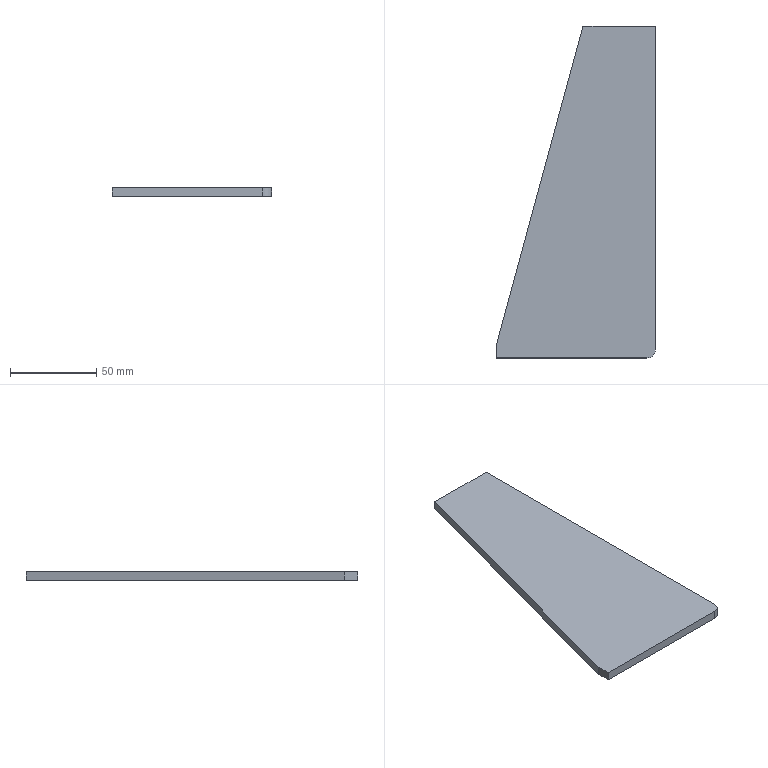Part | SolidWorks | features Extrusion 1 | 1 solid | 8 faces | box 92 x 192 x 5 mm | volume 65293 mm3 | plane 7 | cylinder 1 | commonest cylinder face diameters 10 x1
STEP:
#1=CARTESIAN_POINT('',(42.,-187.,0.));
#2=VERTEX_POINT('',#1);
#3=CARTESIAN_POINT('',(42.,0.,0.));
#4=VERTEX_POINT('',#3);
#5=CARTESIAN_POINT('',(42.,-187.,0.));
#6=DIRECTION('',(0.,1.,0.));
#7=VECTOR('',#6,1000.);
#8=LINE('',#5,#7);
#9=EDGE_CURVE('',#2,#4,#8,.T.);
#10=ORIENTED_EDGE('',*,*,#9,.T.);
#11=CARTESIAN_POINT('',(42.,0.,5.));
#12=VERTEX_POINT('',#11);
#13=CARTESIAN_POINT('',(42.,0.,5.));
#14=DIRECTION('',(0.,0.,-1.));
#15=VECTOR('',#14,1000.);
#16=LINE('',#13,#15);
#17=EDGE_CURVE('',#12,#4,#16,.T.);
#18=ORIENTED_EDGE('',*,*,#17,.F.);
#19=CARTESIAN_POINT('',(42.,-187.,5.));
#20=VERTEX_POINT('',#19);
#21=CARTESIAN_POINT('',(42.,-187.,5.));
#22=DIRECTION('',(0.,1.,0.));
#23=VECTOR('',#22,1000.);
#24=LINE('',#21,#23);
#25=EDGE_CURVE('',#20,#12,#24,.T.);
#26=ORIENTED_EDGE('',*,*,#25,.F.);
#27=CARTESIAN_POINT('',(42.,-187.,5.));
#28=DIRECTION('',(0.,0.,-1.));
#29=VECTOR('',#28,1000.);
#30=LINE('',#27,#29);
#31=EDGE_CURVE('',#20,#2,#30,.T.);
#32=ORIENTED_EDGE('',*,*,#31,.T.);
#33=EDGE_LOOP('',(#10,#18,#26,#32));
#34=FACE_OUTER_BOUND('',#33,.T.);
#35=CARTESIAN_POINT('',(42.,-187.,5.));
#36=DIRECTION('',(-1.,0.,0.));
#37=DIRECTION('',(0.,0.,1.));
#38=AXIS2_PLACEMENT_3D('',#35,#36,#37);
#39=PLANE('',#38);
#40=ADVANCED_FACE('',(#34),#39,.F.);
#41=CARTESIAN_POINT('',(0.,0.,0.));
#42=VERTEX_POINT('',#41);
#43=CARTESIAN_POINT('',(42.,0.,0.));
#44=DIRECTION('',(-1.,0.,0.));
#45=VECTOR('',#44,1000.);
#46=LINE('',#43,#45);
#47=EDGE_CURVE('',#4,#42,#46,.T.);
#48=ORIENTED_EDGE('',*,*,#47,.T.);
#49=CARTESIAN_POINT('',(0.,0.,5.));
#50=VERTEX_POINT('',#49);
#51=CARTESIAN_POINT('',(0.,0.,5.));
#52=DIRECTION('',(0.,0.,-1.));
#53=VECTOR('',#52,1000.);
#54=LINE('',#51,#53);
#55=EDGE_CURVE('',#50,#42,#54,.T.);
#56=ORIENTED_EDGE('',*,*,#55,.F.);
#57=CARTESIAN_POINT('',(42.,0.,5.));
#58=DIRECTION('',(-1.,0.,0.));
#59=VECTOR('',#58,1000.);
#60=LINE('',#57,#59);
#61=EDGE_CURVE('',#12,#50,#60,.T.);
#62=ORIENTED_EDGE('',*,*,#61,.F.);
#63=ORIENTED_EDGE('',*,*,#17,.T.);
#64=EDGE_LOOP('',(#48,#56,#62,#63));
#65=FACE_OUTER_BOUND('',#64,.T.);
#66=CARTESIAN_POINT('',(42.,0.,5.));
#67=DIRECTION('',(0.,-1.,0.));
#68=DIRECTION('',(0.,0.,-1.));
#69=AXIS2_PLACEMENT_3D('',#66,#67,#68);
#70=PLANE('',#69);
#71=ADVANCED_FACE('',(#65),#70,.F.);
#72=CARTESIAN_POINT('',(-50.,-184.,0.));
#73=VERTEX_POINT('',#72);
#74=CARTESIAN_POINT('',(0.,0.,0.));
#75=DIRECTION('',(-0.2622,-0.965,0.));
#76=VECTOR('',#75,1000.);
#77=LINE('',#74,#76);
#78=EDGE_CURVE('',#42,#73,#77,.T.);
#79=ORIENTED_EDGE('',*,*,#78,.T.);
#80=CARTESIAN_POINT('',(-50.,-184.,5.));
#81=VERTEX_POINT('',#80);
#82=CARTESIAN_POINT('',(-50.,-184.,5.));
#83=DIRECTION('',(0.,0.,-1.));
#84=VECTOR('',#83,1000.);
#85=LINE('',#82,#84);
#86=EDGE_CURVE('',#81,#73,#85,.T.);
#87=ORIENTED_EDGE('',*,*,#86,.F.);
#88=CARTESIAN_POINT('',(0.,0.,5.));
#89=DIRECTION('',(-0.2622,-0.965,0.));
#90=VECTOR('',#89,1000.);
#91=LINE('',#88,#90);
#92=EDGE_CURVE('',#50,#81,#91,.T.);
#93=ORIENTED_EDGE('',*,*,#92,.F.);
#94=ORIENTED_EDGE('',*,*,#55,.T.);
#95=EDGE_LOOP('',(#79,#87,#93,#94));
#96=FACE_OUTER_BOUND('',#95,.T.);
#97=CARTESIAN_POINT('',(0.,0.,5.));
#98=DIRECTION('',(0.965,-0.2622,0.));
#99=DIRECTION('',(0.2622,0.965,0.));
#100=AXIS2_PLACEMENT_3D('',#97,#98,#99);
#101=PLANE('',#100);
#102=ADVANCED_FACE('',(#96),#101,.F.);
#103=CARTESIAN_POINT('',(-50.,-192.,0.));
#104=VERTEX_POINT('',#103);
#105=CARTESIAN_POINT('',(-50.,-184.,0.));
#106=DIRECTION('',(0.,-1.,0.));
#107=VECTOR('',#106,1000.);
#108=LINE('',#105,#107);
#109=EDGE_CURVE('',#73,#104,#108,.T.);
#110=ORIENTED_EDGE('',*,*,#109,.T.);
#111=CARTESIAN_POINT('',(-50.,-192.,5.));
#112=VERTEX_POINT('',#111);
#113=CARTESIAN_POINT('',(-50.,-192.,5.));
#114=DIRECTION('',(0.,0.,-1.));
#115=VECTOR('',#114,1000.);
#116=LINE('',#113,#115);
#117=EDGE_CURVE('',#112,#104,#116,.T.);
#118=ORIENTED_EDGE('',*,*,#117,.F.);
#119=CARTESIAN_POINT('',(-50.,-184.,5.));
#120=DIRECTION('',(0.,-1.,0.));
#121=VECTOR('',#120,1000.);
#122=LINE('',#119,#121);
#123=EDGE_CURVE('',#81,#112,#122,.T.);
#124=ORIENTED_EDGE('',*,*,#123,.F.);
#125=ORIENTED_EDGE('',*,*,#86,.T.);
#126=EDGE_LOOP('',(#110,#118,#124,#125));
#127=FACE_OUTER_BOUND('',#126,.T.);
#128=CARTESIAN_POINT('',(-50.,-184.,5.));
#129=DIRECTION('',(1.,0.,0.));
#130=DIRECTION('',(0.,0.,-1.));
#131=AXIS2_PLACEMENT_3D('',#128,#129,#130);
#132=PLANE('',#131);
#133=ADVANCED_FACE('',(#127),#132,.F.);
#134=CARTESIAN_POINT('',(37.,-192.,0.));
#135=VERTEX_POINT('',#134);
#136=CARTESIAN_POINT('',(-50.,-192.,0.));
#137=DIRECTION('',(1.,0.,0.));
#138=VECTOR('',#137,1000.);
#139=LINE('',#136,#138);
#140=EDGE_CURVE('',#104,#135,#139,.T.);
#141=ORIENTED_EDGE('',*,*,#140,.T.);
#142=CARTESIAN_POINT('',(37.,-192.,5.));
#143=VERTEX_POINT('',#142);
#144=CARTESIAN_POINT('',(37.,-192.,5.));
#145=DIRECTION('',(0.,0.,-1.));
#146=VECTOR('',#145,1000.);
#147=LINE('',#144,#146);
#148=EDGE_CURVE('',#143,#135,#147,.T.);
#149=ORIENTED_EDGE('',*,*,#148,.F.);
#150=CARTESIAN_POINT('',(-50.,-192.,5.));
#151=DIRECTION('',(1.,0.,0.));
#152=VECTOR('',#151,1000.);
#153=LINE('',#150,#152);
#154=EDGE_CURVE('',#112,#143,#153,.T.);
#155=ORIENTED_EDGE('',*,*,#154,.F.);
#156=ORIENTED_EDGE('',*,*,#117,.T.);
#157=EDGE_LOOP('',(#141,#149,#155,#156));
#158=FACE_OUTER_BOUND('',#157,.T.);
#159=CARTESIAN_POINT('',(-50.,-192.,5.));
#160=DIRECTION('',(0.,1.,0.));
#161=DIRECTION('',(0.,0.,1.));
#162=AXIS2_PLACEMENT_3D('',#159,#160,#161);
#163=PLANE('',#162);
#164=ADVANCED_FACE('',(#158),#163,.F.);
#165=CARTESIAN_POINT('',(37.,-187.,0.));
#166=DIRECTION('',(0.,0.,1.));
#167=DIRECTION('',(1.,0.,0.));
#168=AXIS2_PLACEMENT_3D('',#165,#166,#167);
#169=CIRCLE('',#168,5.);
#170=EDGE_CURVE('',#135,#2,#169,.T.);
#171=ORIENTED_EDGE('',*,*,#170,.T.);
#172=ORIENTED_EDGE('',*,*,#31,.F.);
#173=CARTESIAN_POINT('',(37.,-187.,5.));
#174=DIRECTION('',(0.,0.,1.));
#175=DIRECTION('',(1.,0.,0.));
#176=AXIS2_PLACEMENT_3D('',#173,#174,#175);
#177=CIRCLE('',#176,5.);
#178=EDGE_CURVE('',#143,#20,#177,.T.);
#179=ORIENTED_EDGE('',*,*,#178,.F.);
#180=ORIENTED_EDGE('',*,*,#148,.T.);
#181=EDGE_LOOP('',(#171,#172,#179,#180));
#182=FACE_OUTER_BOUND('',#181,.T.);
#183=CARTESIAN_POINT('',(37.,-187.,5.));
#184=DIRECTION('',(0.,0.,-1.));
#185=DIRECTION('',(-1.,0.,0.));
#186=AXIS2_PLACEMENT_3D('',#183,#184,#185);
#187=CYLINDRICAL_SURFACE('',#186,5.);
#188=ADVANCED_FACE('',(#182),#187,.T.);
#189=ORIENTED_EDGE('',*,*,#25,.T.);
#190=ORIENTED_EDGE('',*,*,#61,.T.);
#191=ORIENTED_EDGE('',*,*,#92,.T.);
#192=ORIENTED_EDGE('',*,*,#123,.T.);
#193=ORIENTED_EDGE('',*,*,#154,.T.);
#194=ORIENTED_EDGE('',*,*,#178,.T.);
#195=EDGE_LOOP('',(#189,#190,#191,#192,#193,#194));
#196=FACE_OUTER_BOUND('',#195,.T.);
#197=CARTESIAN_POINT('',(37.,-187.,5.));
#198=DIRECTION('',(0.,0.,1.));
#199=DIRECTION('',(1.,0.,0.));
#200=AXIS2_PLACEMENT_3D('',#197,#198,#199);
#201=PLANE('',#200);
#202=ADVANCED_FACE('',(#196),#201,.T.);
#203=ORIENTED_EDGE('',*,*,#9,.F.);
#204=ORIENTED_EDGE('',*,*,#170,.F.);
#205=ORIENTED_EDGE('',*,*,#140,.F.);
#206=ORIENTED_EDGE('',*,*,#109,.F.);
#207=ORIENTED_EDGE('',*,*,#78,.F.);
#208=ORIENTED_EDGE('',*,*,#47,.F.);
#209=EDGE_LOOP('',(#203,#204,#205,#206,#207,#208));
#210=FACE_OUTER_BOUND('',#209,.T.);
#211=CARTESIAN_POINT('',(37.,-187.,0.));
#212=DIRECTION('',(0.,0.,1.));
#213=DIRECTION('',(1.,0.,0.));
#214=AXIS2_PLACEMENT_3D('',#211,#212,#213);
#215=PLANE('',#214);
#216=ADVANCED_FACE('',(#210),#215,.F.);
#217=CLOSED_SHELL('',(#40,#71,#102,#133,#164,#188,#202,#216));
#218=MANIFOLD_SOLID_BREP('',#217);
#219=CARTESIAN_POINT('',(0.,0.,0.));
#220=DIRECTION('',(0.,0.,1.));
#221=DIRECTION('',(1.,0.,0.));
#222=AXIS2_PLACEMENT_3D('',#219,#220,#221);
#223=(LENGTH_UNIT()NAMED_UNIT(*)SI_UNIT(.MILLI.,.METRE.));
#224=UNCERTAINTY_MEASURE_WITH_UNIT(LENGTH_MEASURE(0.00001),#223,'','');
#225=(NAMED_UNIT(*)PLANE_ANGLE_UNIT()SI_UNIT($,.RADIAN.));
#226=(NAMED_UNIT(*)SI_UNIT($,.STERADIAN.)SOLID_ANGLE_UNIT());
#227=(GEOMETRIC_REPRESENTATION_CONTEXT(3)GLOBAL_UNCERTAINTY_ASSIGNED_CONTEXT((#224))GLOBAL_UNIT_ASSIGNED_CONTEXT((#223,#225,#226))REPRESENTATION_CONTEXT('',''));
#228=ADVANCED_BREP_SHAPE_REPRESENTATION('',(#218,#222),#227);